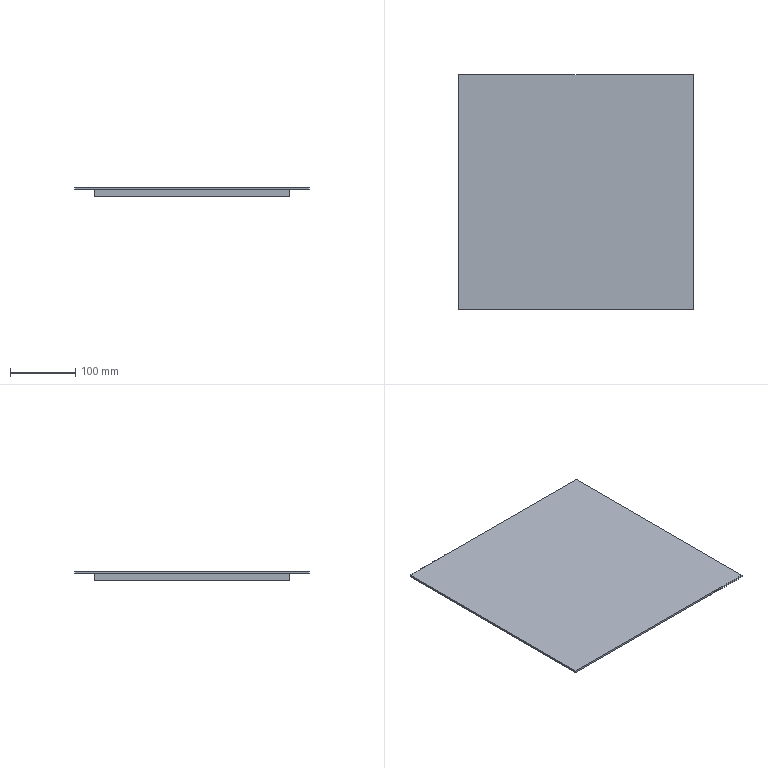Part | STEP file | 750038251 | 1 solid | 11 faces | box 360 x 360 x 15 mm | volume 1468800 mm3 | plane 11
STEP:
#1=CARTESIAN_POINT('',(180.,-180.,15.));
#2=VERTEX_POINT('',#1);
#3=CARTESIAN_POINT('',(180.,180.,15.));
#4=VERTEX_POINT('',#3);
#5=CARTESIAN_POINT('',(180.,0.,15.));
#6=DIRECTION('',(0.,1.,0.));
#7=VECTOR('',#6,1000.);
#8=LINE('',#5,#7);
#9=EDGE_CURVE('',#2,#4,#8,.T.);
#10=ORIENTED_EDGE('',*,*,#9,.T.);
#11=CARTESIAN_POINT('',(-180.,180.,15.));
#12=VERTEX_POINT('',#11);
#13=CARTESIAN_POINT('',(0.,180.,15.));
#14=DIRECTION('',(-1.,0.,0.));
#15=VECTOR('',#14,1000.);
#16=LINE('',#13,#15);
#17=EDGE_CURVE('',#4,#12,#16,.T.);
#18=ORIENTED_EDGE('',*,*,#17,.T.);
#19=CARTESIAN_POINT('',(-180.,-180.,15.));
#20=VERTEX_POINT('',#19);
#21=CARTESIAN_POINT('',(-180.,0.,15.));
#22=DIRECTION('',(0.,-1.,0.));
#23=VECTOR('',#22,1000.);
#24=LINE('',#21,#23);
#25=EDGE_CURVE('',#12,#20,#24,.T.);
#26=ORIENTED_EDGE('',*,*,#25,.T.);
#27=CARTESIAN_POINT('',(0.,-180.,15.));
#28=DIRECTION('',(1.,0.,0.));
#29=VECTOR('',#28,1000.);
#30=LINE('',#27,#29);
#31=EDGE_CURVE('',#20,#2,#30,.T.);
#32=ORIENTED_EDGE('',*,*,#31,.T.);
#33=EDGE_LOOP('',(#10,#18,#26,#32));
#34=FACE_OUTER_BOUND('',#33,.T.);
#35=CARTESIAN_POINT('',(0.,0.,15.));
#36=DIRECTION('',(0.,0.,1.));
#37=DIRECTION('',(1.,0.,0.));
#38=AXIS2_PLACEMENT_3D('',#35,#36,#37);
#39=PLANE('',#38);
#40=ADVANCED_FACE('',(#34),#39,.T.);
#41=CARTESIAN_POINT('',(180.,180.,12.));
#42=VERTEX_POINT('',#41);
#43=CARTESIAN_POINT('',(-180.,180.,12.));
#44=VERTEX_POINT('',#43);
#45=CARTESIAN_POINT('',(180.,180.,12.));
#46=DIRECTION('',(-1.,0.,0.));
#47=VECTOR('',#46,1000.);
#48=LINE('',#45,#47);
#49=EDGE_CURVE('',#42,#44,#48,.T.);
#50=ORIENTED_EDGE('',*,*,#49,.T.);
#51=CARTESIAN_POINT('',(-180.,180.,12.));
#52=DIRECTION('',(0.,0.,1.));
#53=VECTOR('',#52,1000.);
#54=LINE('',#51,#53);
#55=EDGE_CURVE('',#44,#12,#54,.T.);
#56=ORIENTED_EDGE('',*,*,#55,.T.);
#57=ORIENTED_EDGE('',*,*,#17,.F.);
#58=CARTESIAN_POINT('',(180.,180.,12.));
#59=DIRECTION('',(0.,0.,-1.));
#60=VECTOR('',#59,1000.);
#61=LINE('',#58,#60);
#62=EDGE_CURVE('',#4,#42,#61,.T.);
#63=ORIENTED_EDGE('',*,*,#62,.T.);
#64=EDGE_LOOP('',(#50,#56,#57,#63));
#65=FACE_OUTER_BOUND('',#64,.T.);
#66=CARTESIAN_POINT('',(180.,180.,12.));
#67=DIRECTION('',(0.,1.,0.));
#68=DIRECTION('',(-1.,0.,0.));
#69=AXIS2_PLACEMENT_3D('',#66,#67,#68);
#70=PLANE('',#69);
#71=ADVANCED_FACE('',(#65),#70,.T.);
#72=CARTESIAN_POINT('',(180.,-180.,12.));
#73=VERTEX_POINT('',#72);
#74=CARTESIAN_POINT('',(180.,-180.,12.));
#75=DIRECTION('',(0.,1.,0.));
#76=VECTOR('',#75,1000.);
#77=LINE('',#74,#76);
#78=EDGE_CURVE('',#73,#42,#77,.T.);
#79=ORIENTED_EDGE('',*,*,#78,.T.);
#80=ORIENTED_EDGE('',*,*,#62,.F.);
#81=ORIENTED_EDGE('',*,*,#9,.F.);
#82=CARTESIAN_POINT('',(180.,-180.,12.));
#83=DIRECTION('',(0.,0.,-1.));
#84=VECTOR('',#83,1000.);
#85=LINE('',#82,#84);
#86=EDGE_CURVE('',#2,#73,#85,.T.);
#87=ORIENTED_EDGE('',*,*,#86,.T.);
#88=EDGE_LOOP('',(#79,#80,#81,#87));
#89=FACE_OUTER_BOUND('',#88,.T.);
#90=CARTESIAN_POINT('',(180.,-180.,12.));
#91=DIRECTION('',(1.,0.,0.));
#92=DIRECTION('',(0.,1.,0.));
#93=AXIS2_PLACEMENT_3D('',#90,#91,#92);
#94=PLANE('',#93);
#95=ADVANCED_FACE('',(#89),#94,.T.);
#96=CARTESIAN_POINT('',(-180.,-180.,12.));
#97=VERTEX_POINT('',#96);
#98=CARTESIAN_POINT('',(-180.,-180.,12.));
#99=DIRECTION('',(1.,0.,0.));
#100=VECTOR('',#99,1000.);
#101=LINE('',#98,#100);
#102=EDGE_CURVE('',#97,#73,#101,.T.);
#103=ORIENTED_EDGE('',*,*,#102,.T.);
#104=ORIENTED_EDGE('',*,*,#86,.F.);
#105=ORIENTED_EDGE('',*,*,#31,.F.);
#106=CARTESIAN_POINT('',(-180.,-180.,12.));
#107=DIRECTION('',(0.,0.,-1.));
#108=VECTOR('',#107,1000.);
#109=LINE('',#106,#108);
#110=EDGE_CURVE('',#20,#97,#109,.T.);
#111=ORIENTED_EDGE('',*,*,#110,.T.);
#112=EDGE_LOOP('',(#103,#104,#105,#111));
#113=FACE_OUTER_BOUND('',#112,.T.);
#114=CARTESIAN_POINT('',(-180.,-180.,12.));
#115=DIRECTION('',(0.,-1.,0.));
#116=DIRECTION('',(0.,0.,-1.));
#117=AXIS2_PLACEMENT_3D('',#114,#115,#116);
#118=PLANE('',#117);
#119=ADVANCED_FACE('',(#113),#118,.T.);
#120=CARTESIAN_POINT('',(-180.,180.,12.));
#121=DIRECTION('',(0.,-1.,0.));
#122=VECTOR('',#121,1000.);
#123=LINE('',#120,#122);
#124=EDGE_CURVE('',#44,#97,#123,.T.);
#125=ORIENTED_EDGE('',*,*,#124,.T.);
#126=ORIENTED_EDGE('',*,*,#110,.F.);
#127=ORIENTED_EDGE('',*,*,#25,.F.);
#128=ORIENTED_EDGE('',*,*,#55,.F.);
#129=EDGE_LOOP('',(#125,#126,#127,#128));
#130=FACE_OUTER_BOUND('',#129,.T.);
#131=CARTESIAN_POINT('',(-180.,180.,12.));
#132=DIRECTION('',(-1.,0.,0.));
#133=DIRECTION('',(0.,-1.,0.));
#134=AXIS2_PLACEMENT_3D('',#131,#132,#133);
#135=PLANE('',#134);
#136=ADVANCED_FACE('',(#130),#135,.T.);
#137=CARTESIAN_POINT('',(150.,-150.,12.));
#138=VERTEX_POINT('',#137);
#139=CARTESIAN_POINT('',(-150.,-150.,12.));
#140=VERTEX_POINT('',#139);
#141=CARTESIAN_POINT('',(0.,-150.,12.));
#142=DIRECTION('',(-1.,0.,0.));
#143=VECTOR('',#142,1000.);
#144=LINE('',#141,#143);
#145=EDGE_CURVE('',#138,#140,#144,.T.);
#146=ORIENTED_EDGE('',*,*,#145,.F.);
#147=CARTESIAN_POINT('',(150.,150.,12.));
#148=VERTEX_POINT('',#147);
#149=CARTESIAN_POINT('',(150.,0.,12.));
#150=DIRECTION('',(0.,-1.,0.));
#151=VECTOR('',#150,1000.);
#152=LINE('',#149,#151);
#153=EDGE_CURVE('',#148,#138,#152,.T.);
#154=ORIENTED_EDGE('',*,*,#153,.F.);
#155=CARTESIAN_POINT('',(-150.,150.,12.));
#156=VERTEX_POINT('',#155);
#157=CARTESIAN_POINT('',(0.,150.,12.));
#158=DIRECTION('',(1.,0.,0.));
#159=VECTOR('',#158,1000.);
#160=LINE('',#157,#159);
#161=EDGE_CURVE('',#156,#148,#160,.T.);
#162=ORIENTED_EDGE('',*,*,#161,.F.);
#163=CARTESIAN_POINT('',(-150.,0.,12.));
#164=DIRECTION('',(0.,1.,0.));
#165=VECTOR('',#164,1000.);
#166=LINE('',#163,#165);
#167=EDGE_CURVE('',#140,#156,#166,.T.);
#168=ORIENTED_EDGE('',*,*,#167,.F.);
#169=EDGE_LOOP('',(#146,#154,#162,#168));
#170=FACE_BOUND('',#169,.T.);
#171=ORIENTED_EDGE('',*,*,#49,.F.);
#172=ORIENTED_EDGE('',*,*,#78,.F.);
#173=ORIENTED_EDGE('',*,*,#102,.F.);
#174=ORIENTED_EDGE('',*,*,#124,.F.);
#175=EDGE_LOOP('',(#171,#172,#173,#174));
#176=FACE_OUTER_BOUND('',#175,.T.);
#177=CARTESIAN_POINT('',(0.,0.,12.));
#178=DIRECTION('',(0.,0.,1.));
#179=DIRECTION('',(1.,0.,0.));
#180=AXIS2_PLACEMENT_3D('',#177,#178,#179);
#181=PLANE('',#180);
#182=ADVANCED_FACE('',(#170,#176),#181,.F.);
#183=ORIENTED_EDGE('',*,*,#167,.T.);
#184=CARTESIAN_POINT('',(-150.,150.,0.));
#185=VERTEX_POINT('',#184);
#186=CARTESIAN_POINT('',(-150.,150.,15.));
#187=DIRECTION('',(0.,0.,1.));
#188=VECTOR('',#187,1000.);
#189=LINE('',#186,#188);
#190=EDGE_CURVE('',#185,#156,#189,.T.);
#191=ORIENTED_EDGE('',*,*,#190,.F.);
#192=CARTESIAN_POINT('',(-150.,-150.,0.));
#193=VERTEX_POINT('',#192);
#194=CARTESIAN_POINT('',(-150.,150.,0.));
#195=DIRECTION('',(0.,1.,0.));
#196=VECTOR('',#195,1000.);
#197=LINE('',#194,#196);
#198=EDGE_CURVE('',#193,#185,#197,.T.);
#199=ORIENTED_EDGE('',*,*,#198,.F.);
#200=CARTESIAN_POINT('',(-150.,-150.,15.));
#201=DIRECTION('',(0.,0.,-1.));
#202=VECTOR('',#201,1000.);
#203=LINE('',#200,#202);
#204=EDGE_CURVE('',#140,#193,#203,.T.);
#205=ORIENTED_EDGE('',*,*,#204,.F.);
#206=EDGE_LOOP('',(#183,#191,#199,#205));
#207=FACE_OUTER_BOUND('',#206,.T.);
#208=CARTESIAN_POINT('',(-150.,150.,15.));
#209=DIRECTION('',(1.,0.,0.));
#210=DIRECTION('',(0.,0.,-1.));
#211=AXIS2_PLACEMENT_3D('',#208,#209,#210);
#212=PLANE('',#211);
#213=ADVANCED_FACE('',(#207),#212,.F.);
#214=ORIENTED_EDGE('',*,*,#145,.T.);
#215=ORIENTED_EDGE('',*,*,#204,.T.);
#216=CARTESIAN_POINT('',(150.,-150.,0.));
#217=VERTEX_POINT('',#216);
#218=CARTESIAN_POINT('',(-150.,-150.,0.));
#219=DIRECTION('',(-1.,0.,0.));
#220=VECTOR('',#219,1000.);
#221=LINE('',#218,#220);
#222=EDGE_CURVE('',#217,#193,#221,.T.);
#223=ORIENTED_EDGE('',*,*,#222,.F.);
#224=CARTESIAN_POINT('',(150.,-150.,15.));
#225=DIRECTION('',(0.,0.,-1.));
#226=VECTOR('',#225,1000.);
#227=LINE('',#224,#226);
#228=EDGE_CURVE('',#138,#217,#227,.T.);
#229=ORIENTED_EDGE('',*,*,#228,.F.);
#230=EDGE_LOOP('',(#214,#215,#223,#229));
#231=FACE_OUTER_BOUND('',#230,.T.);
#232=CARTESIAN_POINT('',(-150.,-150.,15.));
#233=DIRECTION('',(0.,1.,0.));
#234=DIRECTION('',(0.,0.,1.));
#235=AXIS2_PLACEMENT_3D('',#232,#233,#234);
#236=PLANE('',#235);
#237=ADVANCED_FACE('',(#231),#236,.F.);
#238=ORIENTED_EDGE('',*,*,#153,.T.);
#239=ORIENTED_EDGE('',*,*,#228,.T.);
#240=CARTESIAN_POINT('',(150.,150.,0.));
#241=VERTEX_POINT('',#240);
#242=CARTESIAN_POINT('',(150.,-150.,0.));
#243=DIRECTION('',(0.,-1.,0.));
#244=VECTOR('',#243,1000.);
#245=LINE('',#242,#244);
#246=EDGE_CURVE('',#241,#217,#245,.T.);
#247=ORIENTED_EDGE('',*,*,#246,.F.);
#248=CARTESIAN_POINT('',(150.,150.,15.));
#249=DIRECTION('',(0.,0.,-1.));
#250=VECTOR('',#249,1000.);
#251=LINE('',#248,#250);
#252=EDGE_CURVE('',#148,#241,#251,.T.);
#253=ORIENTED_EDGE('',*,*,#252,.F.);
#254=EDGE_LOOP('',(#238,#239,#247,#253));
#255=FACE_OUTER_BOUND('',#254,.T.);
#256=CARTESIAN_POINT('',(150.,-150.,15.));
#257=DIRECTION('',(-1.,0.,0.));
#258=DIRECTION('',(0.,0.,1.));
#259=AXIS2_PLACEMENT_3D('',#256,#257,#258);
#260=PLANE('',#259);
#261=ADVANCED_FACE('',(#255),#260,.F.);
#262=ORIENTED_EDGE('',*,*,#161,.T.);
#263=ORIENTED_EDGE('',*,*,#252,.T.);
#264=CARTESIAN_POINT('',(150.,150.,0.));
#265=DIRECTION('',(1.,0.,0.));
#266=VECTOR('',#265,1000.);
#267=LINE('',#264,#266);
#268=EDGE_CURVE('',#185,#241,#267,.T.);
#269=ORIENTED_EDGE('',*,*,#268,.F.);
#270=ORIENTED_EDGE('',*,*,#190,.T.);
#271=EDGE_LOOP('',(#262,#263,#269,#270));
#272=FACE_OUTER_BOUND('',#271,.T.);
#273=CARTESIAN_POINT('',(150.,150.,15.));
#274=DIRECTION('',(0.,-1.,0.));
#275=DIRECTION('',(0.,0.,-1.));
#276=AXIS2_PLACEMENT_3D('',#273,#274,#275);
#277=PLANE('',#276);
#278=ADVANCED_FACE('',(#272),#277,.F.);
#279=ORIENTED_EDGE('',*,*,#246,.T.);
#280=ORIENTED_EDGE('',*,*,#222,.T.);
#281=ORIENTED_EDGE('',*,*,#198,.T.);
#282=ORIENTED_EDGE('',*,*,#268,.T.);
#283=EDGE_LOOP('',(#279,#280,#281,#282));
#284=FACE_OUTER_BOUND('',#283,.T.);
#285=CARTESIAN_POINT('',(0.,0.,0.));
#286=DIRECTION('',(0.,0.,1.));
#287=DIRECTION('',(1.,0.,0.));
#288=AXIS2_PLACEMENT_3D('',#285,#286,#287);
#289=PLANE('',#288);
#290=ADVANCED_FACE('',(#284),#289,.F.);
#291=CLOSED_SHELL('',(#40,#71,#95,#119,#136,#182,#213,#237,#261,#278,#290));
#292=MANIFOLD_SOLID_BREP('',#291);
#293=CARTESIAN_POINT('',(0.,0.,0.));
#294=DIRECTION('',(0.,0.,1.));
#295=DIRECTION('',(1.,0.,0.));
#296=AXIS2_PLACEMENT_3D('',#293,#294,#295);
#297=(LENGTH_UNIT()NAMED_UNIT(*)SI_UNIT(.MILLI.,.METRE.));
#298=UNCERTAINTY_MEASURE_WITH_UNIT(LENGTH_MEASURE(0.00001),#297,'','');
#299=(NAMED_UNIT(*)PLANE_ANGLE_UNIT()SI_UNIT($,.RADIAN.));
#300=(NAMED_UNIT(*)SI_UNIT($,.STERADIAN.)SOLID_ANGLE_UNIT());
#301=(GEOMETRIC_REPRESENTATION_CONTEXT(3)GLOBAL_UNCERTAINTY_ASSIGNED_CONTEXT((#298))GLOBAL_UNIT_ASSIGNED_CONTEXT((#297,#299,#300))REPRESENTATION_CONTEXT('',''));
#302=ADVANCED_BREP_SHAPE_REPRESENTATION('',(#292,#296),#301);